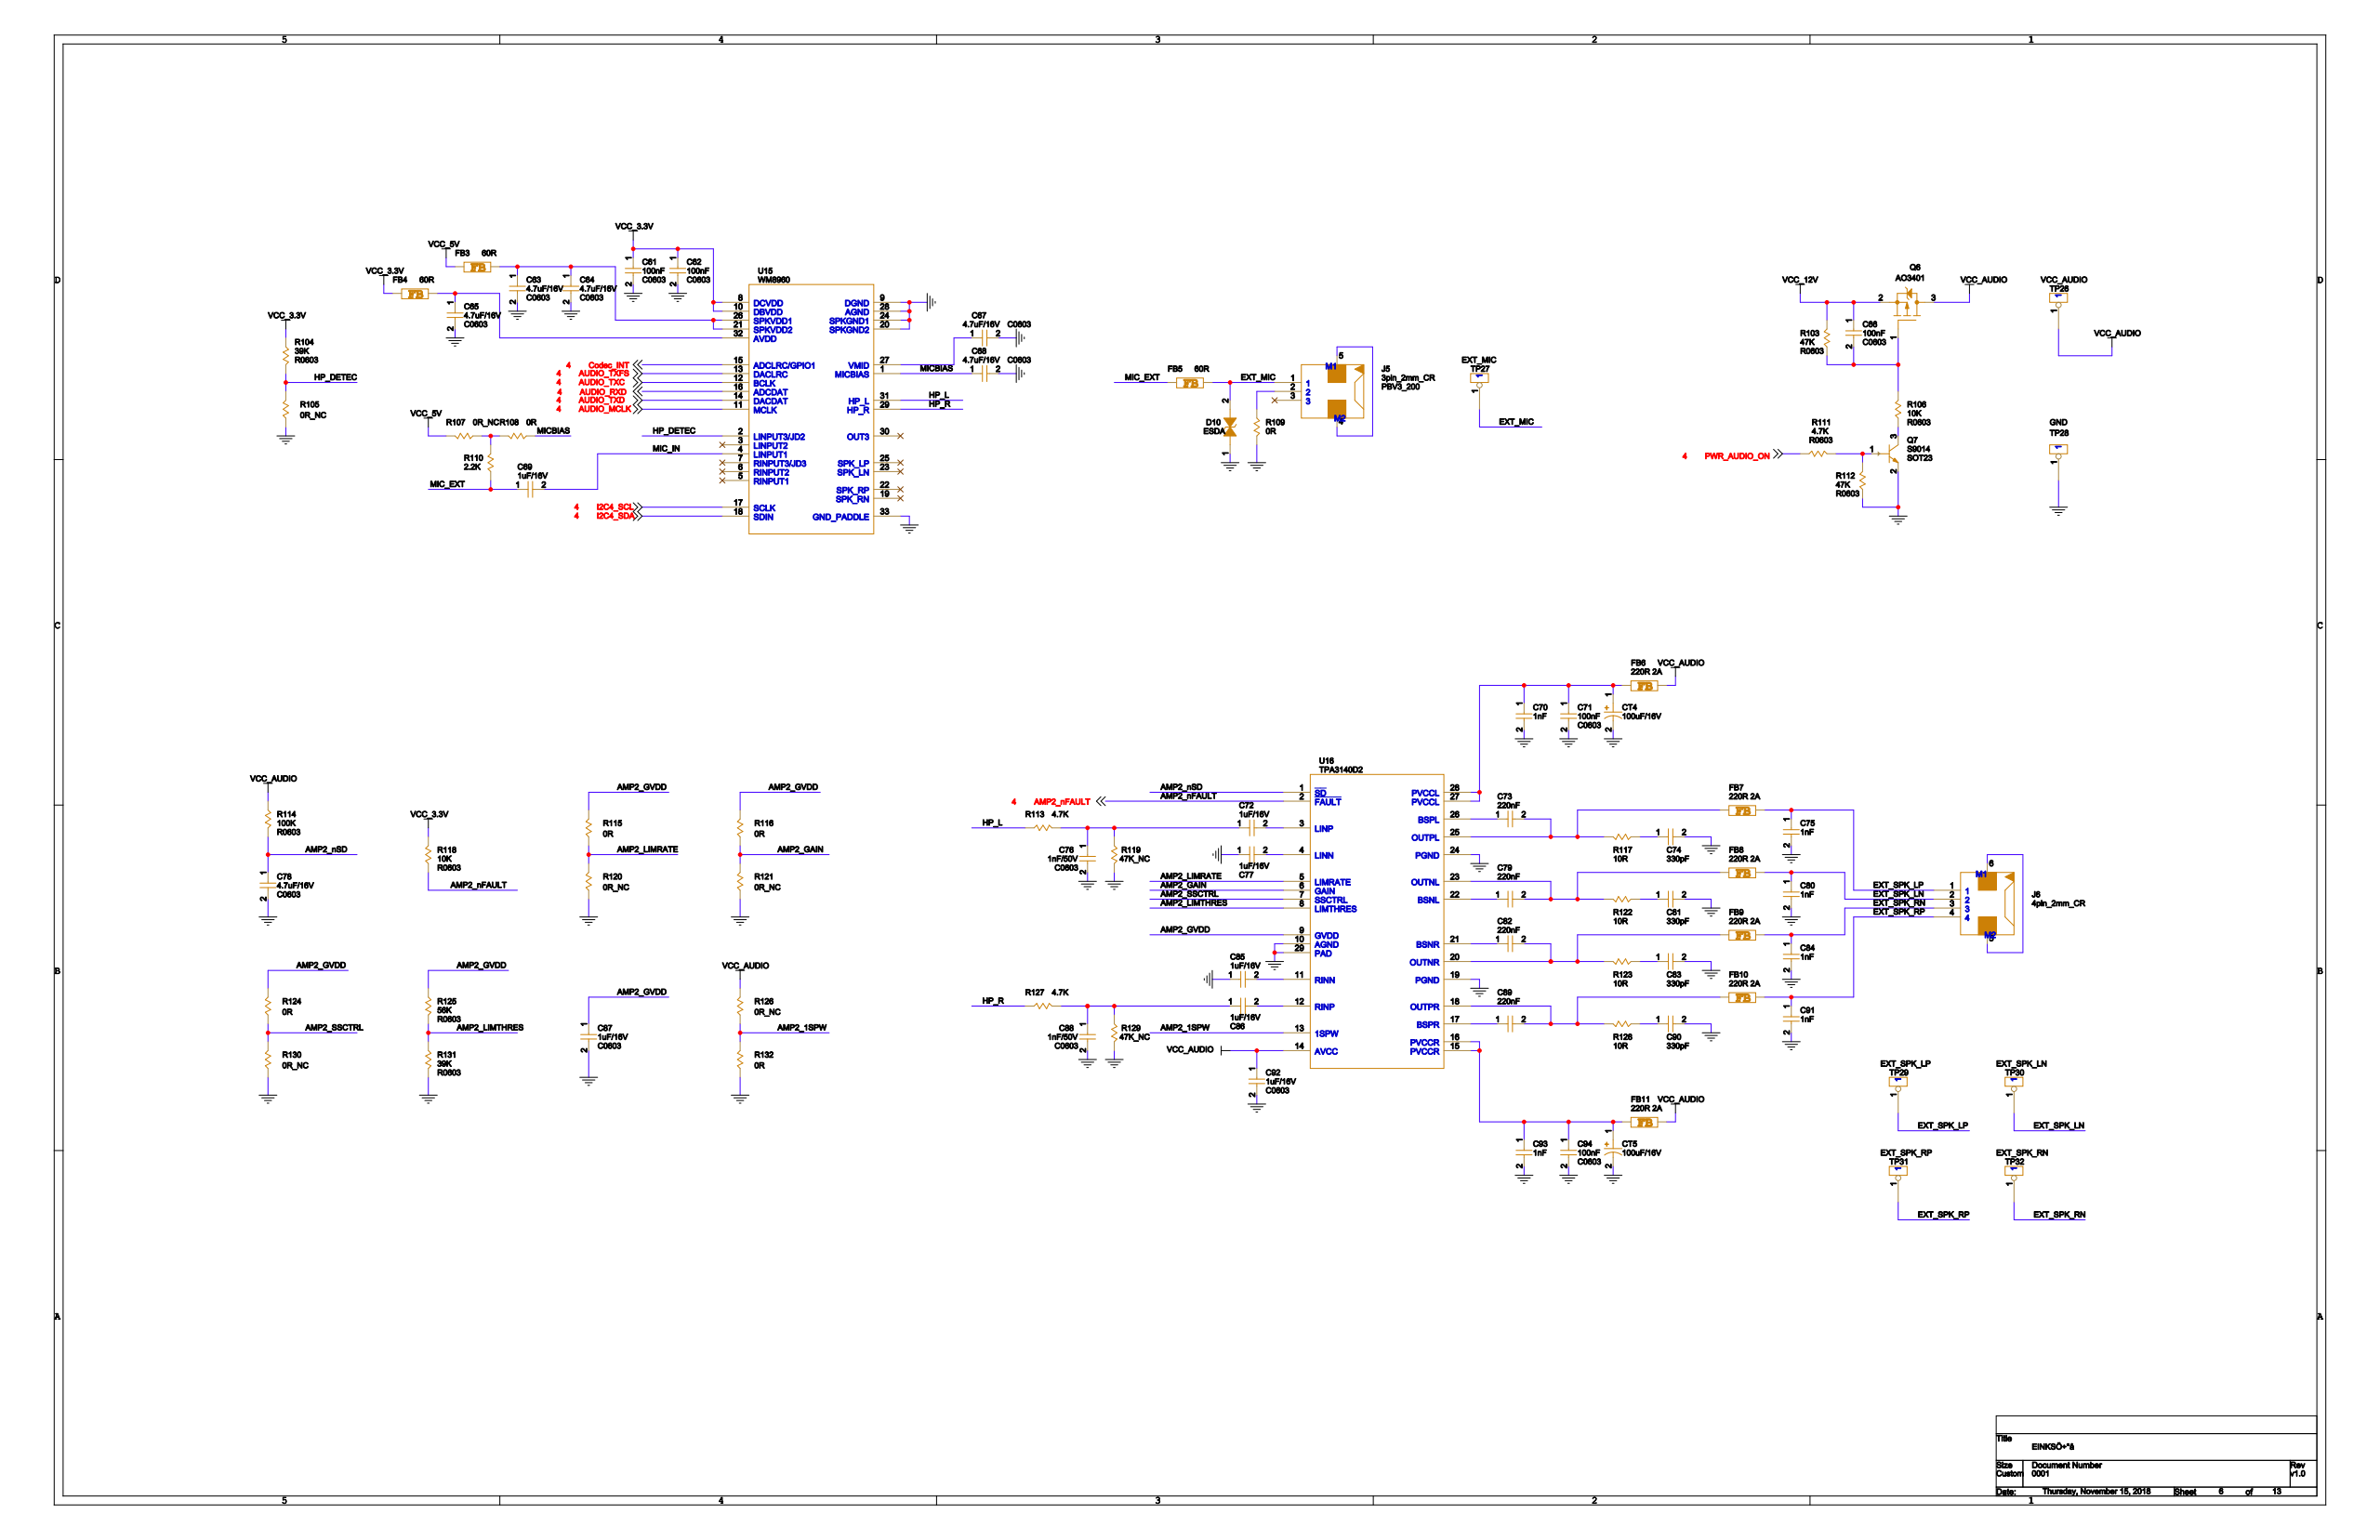Circuit board | Cadence Allegro | 609 parts | 409 nets | one sheet of the schematic
Parts on this sheet (reference | value | footprint):
C61 | 100nF | C0603
C62 | 100nF | C0603
C63 | 4.7uF/16V | C0603
C64 | 4.7uF/16V | C0603
C65 | 4.7uF/16V | C0603
C66 | 100nF | C0603
C67 | 4.7uF/16V | C0603
C68 | 4.7uF/16V | C0603
C69 | 1uF/16V | C0603
C70 | 1nF | C0603
C71 | 100nF | C0603
C72 | 1uF/16V | C0603
C73 | 220nF | C0603
C74 | 330pF | C0603
C75 | 1nF | C0603
C76 | 1nF/50V | C0603
C77 | 1uF/16V | C0603
C78 | 4.7uF/16V | C0603
C79 | 220nF | C0603
C80 | 1nF | C0603
C81 | 330pF | C0603
C82 | 220nF | C0603
C83 | 330pF | C0603
C84 | 1nF | C0603
C85 | 1uF/16V | C0603
C86 | 1uF/16V | C0603
C87 | 1uF/16V | C0603
C88 | 1nF/50V | C0603
C89 | 220nF | C0603
C90 | 330pF | C0603
C91 | 1nF | C0603
C92 | 1uF/16V | C0603
C93 | 1nF | C0603
C94 | 100nF | C0603
CT4 | 100uF/16V | D_CASE
CT5 | 100uF/16V | D_CASE
D10 | ESDA | 0603ESDA
FB3 | 60R | FB0603
FB4 | 60R | FB0603
FB5 | 60R | FB0603
FB6 | 220R 2A | FB0805
FB7 | 220R 2A | FB0805
FB8 | 220R 2A | FB0805
FB9 | 220R 2A | FB0805
FB10 | 220R 2A | FB0805
FB11 | 220R 2A | FB0805
J5 | 3pin_2mm_CR | PBV3_200
J6 | 4pin_2mm_CR | PBV4_200
Q6 | AO3401 | SOT23
Q7 | S9014 | SOT23
R103 | 47K | R0603
R104 | 39K | R0603
R105 | 0R_NC | R0603
R106 | 10K | R0603
R107 | 0R_NC | R0603
R109 | 0R | R0603
R110 | 2.2K | R0603
R111 | 4.7K | R0603
R112 | 47K | R0603
R113 | 4.7K | R0603
R114 | 100K | R0603
R115 | 0R | R0603
R116 | 0R | R0603
R117 | 10R | R0603
R118 | 10K | R0603
R119 | 47K_NC | R0603
R120 | 0R_NC | R0603
R121 | 0R_NC | R0603
R122 | 10R | R0603
R123 | 10R | R0603
R124 | 0R | R0603
R125 | 56K | R0603
R126 | 0R_NC | R0603
R127 | 4.7K | R0603
R128 | 10R | R0603
R129 | 47K_NC | R0603
R130 | 0R_NC | R0603
R131 | 39K | R0603
R132 | 0R | R0603
TP26 | VCC_AUDIO | TP_50
TP27 | EXT_MIC | TP_50
TP28 | GND | TP_50
TP29 | EXT_SPK_LP | TP_50
TP30 | EXT_SPK_LN | TP_50
TP31 | EXT_SPK_RP | TP_50
TP32 | EXT_SPK_RN | TP_50
U15 | WM8960 | QFN32P
U16 | TPA3140D2 | HTSSOP28
Nets of these parts (net: part-pin ...):
GND: C61-2 C62-2 C63-2 C64-2 C65-2 C67-2 C68-2 C70-2 C71-2 C74-2 C75-2 C76-2 C77-1 C78-2 C80-2 C81-2 C83-2 C84-2 C85-1 C87-2 C88-2 C90-2 C91-2 C92-2 C93-2 C94-2 CT4-2 CT5-2 D10-1 Q7-2 R105-2 R109-1 R112-2 R119-2 R120-2 R121-2 R129-2 R130-2 R131-2 R132-2 TP28-1 U15-9 U15-20 U15-24 U15-28 U15-33 U16-10 U16-19 U16-24 U16-29
VCC_12V: C66-1 Q6-2 R103-1
VCC_3.3V: C61-1 C62-1 FB4-1 R104-1 R118-2 U15-8 U15-10
VCC_5V: FB3-1 R107-1
N27961516: C70-1 C71-1 CT4-1 FB6-1 U16-27 U16-28
N27962440: C93-1 C94-1 CT5-1 FB11-1 U16-15 U16-16
EXT_MIC: D10-2 FB5-2 J5-1 TP27-1
N28832298: C63-1 C64-1 FB3-2 U15-21 U15-26
N28833843: C65-1 FB4-2 U15-32
MIC_EXT: C69-1 FB5-1 R110-2
N28854924: J5-2 R109-2
N28852538: J5-4 J5-5
AUDIO_MCLK: U15-11
AUDIO_RXD: U15-16
AUDIO_TXC: U15-12
AUDIO_TXD: U15-14
AUDIO_TXFS: U15-13
I2C4_SCL: U15-17
I2C4_SDA: U15-18
AMP2_NFAULT: R118-1 U16-2
PWR_AUDIO_ON: R111-2
EXT_SPK_LP: C75-1 FB7-2 J6-1 TP29-1
EXT_SPK_LN: C80-1 FB8-2 J6-2 TP30-1
EXT_SPK_RN: C84-1 FB9-2 J6-3 TP32-1
EXT_SPK_RP: C91-1 FB10-2 J6-4 TP31-1
N28868753: J6-5 J6-6
HP_DETEC: R104-2 R105-1 U15-2
AMP2_LIMTHRES: R125-2 R131-1 U16-8
VCC_AUDIO: C92-1 FB6-2 FB11-2 Q6-3 R114-2 R126-1 TP26-1 U16-14
HP_L: R113-2 U15-31
HP_R: R127-2 U15-29
MIC_IN: C69-2 U15-4
MICBIAS: C68-1 U15-1
N28847118: C67-1 U15-27
AMP2_1SPW: R126-2 R132-1 U16-13
N27973262: C79-1 U16-22
N27975795: C82-1 U16-21
N27971458: C73-1 U16-26
N27976315: C89-1 U16-17
AMP2_GAIN: R116-2 R121-1 U16-6
AMP2_GVDD: C87-1 R115-1 R116-1 R124-1 R125-1 U16-9
AMP2_LIMRATE: R115-2 R120-1 U16-5
N27978282: C77-2 U16-4
N27978295: C72-2 U16-3
N27973025: C79-2 FB8-1 R122-2 U16-23
N27973338: C82-2 FB9-1 R123-2 U16-20
N27967850: C73-2 FB7-1 R117-2 U16-25
N27976156: C89-2 FB10-1 R128-2 U16-18
N27978578: C85-2 U16-11
N27979192: C86-2 U16-12
AMP2_SSCTRL: R124-2 R130-1 U16-7
AMP2_NSD: C78-1 R114-1 U16-1
N28004675: C72-1 C76-1 R113-1 R119-1
N27997543: C86-1 C88-1 R127-1 R129-1
N27967942: C74-1 R117-1
N27973027: C81-1 R122-1
N27973348: C83-1 R123-1
N27976170: C90-1 R128-1
N28128162: C66-2 Q6-1 R103-2 R106-2
N28128116: Q7-1 R111-1 R112-1
N28128180: Q7-3 R106-1
N28838347: R107-2 R110-1